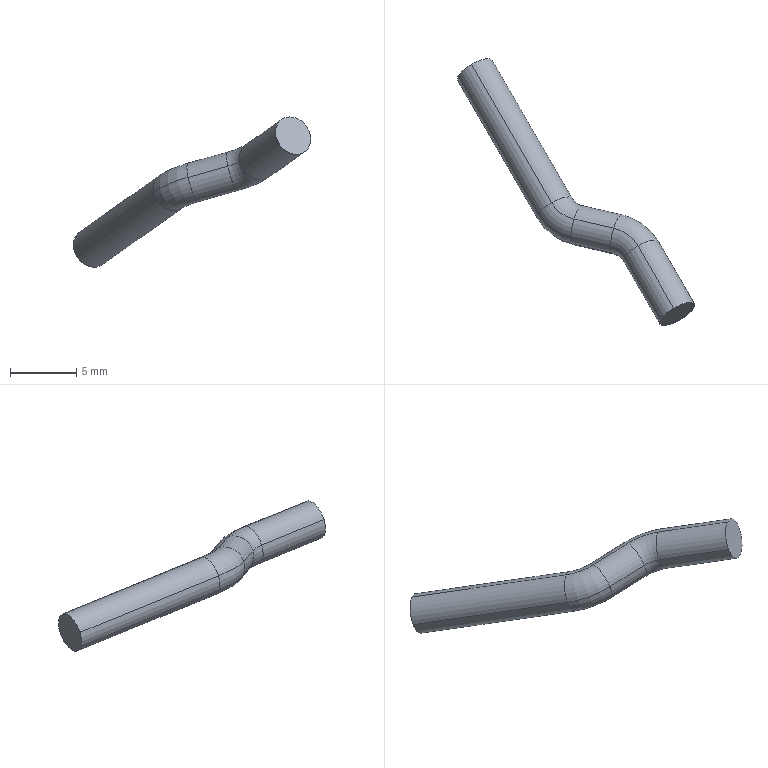Part | STEP file | MSBR-16_1_5_4_2_1 | 1 solid | 17 faces | box 17.856 x 20.083 x 11.306 mm | volume 186.454 mm3 | cylinder 9 | torus 6 | plane 2 | commonest cylinder face diameters 3 x9
STEP:
#1=CARTESIAN_POINT('',(0.,0.,0.));
#2=DIRECTION('',(0.,0.,1.));
#3=DIRECTION('',(1.,0.,0.));
#4=AXIS2_PLACEMENT_3D('',#1,#2,#3);
#5=CARTESIAN_POINT('',(6.735,-43.041,129.068));
#6=VERTEX_POINT('',#5);
#7=CARTESIAN_POINT('',(7.784,-41.858,130.482));
#8=VERTEX_POINT('',#7);
#9=CARTESIAN_POINT('',(8.034,-42.291,129.068));
#10=DIRECTION('',(-0.4714,0.8165,-0.3333));
#11=DIRECTION('',(-0.866,-0.5,-0.00009773));
#12=AXIS2_PLACEMENT_3D('',#9,#10,#11);
#13=CIRCLE('',#12,1.5);
#14=EDGE_CURVE('',#6,#8,#13,.T.);
#15=ORIENTED_EDGE('',*,*,#14,.F.);
#16=CARTESIAN_POINT('',(0.7209,-32.624,124.815));
#17=VERTEX_POINT('',#16);
#18=CARTESIAN_POINT('',(0.7209,-32.624,124.815));
#19=DIRECTION('',(0.4714,-0.8165,0.3333));
#20=VECTOR('',#19,12.757);
#21=LINE('',#18,#20);
#22=EDGE_CURVE('',#17,#6,#21,.T.);
#23=ORIENTED_EDGE('',*,*,#22,.F.);
#24=CARTESIAN_POINT('',(1.77,-31.441,126.23));
#25=VERTEX_POINT('',#24);
#26=CARTESIAN_POINT('',(2.02,-31.874,124.816));
#27=DIRECTION('',(0.4714,-0.8165,0.3333));
#28=DIRECTION('',(-0.1666,0.2887,0.9428));
#29=AXIS2_PLACEMENT_3D('',#26,#27,#28);
#30=CIRCLE('',#29,1.5);
#31=EDGE_CURVE('',#25,#17,#30,.T.);
#32=ORIENTED_EDGE('',*,*,#31,.F.);
#33=CARTESIAN_POINT('',(7.784,-41.858,130.482));
#34=DIRECTION('',(-0.4714,0.8165,-0.3333));
#35=VECTOR('',#34,12.757);
#36=LINE('',#33,#35);
#37=EDGE_CURVE('',#8,#25,#36,.T.);
#38=ORIENTED_EDGE('',*,*,#37,.F.);
#39=EDGE_LOOP('',(#15,#23,#32,#38));
#40=FACE_OUTER_BOUND('',#39,.F.);
#41=CARTESIAN_POINT('',(8.034,-42.291,129.068));
#42=DIRECTION('',(0.4714,-0.8165,0.3333));
#43=DIRECTION('',(-0.1668,0.2886,0.9428));
#44=AXIS2_PLACEMENT_3D('',#41,#42,#43);
#45=CYLINDRICAL_SURFACE('',#44,1.5);
#46=ADVANCED_FACE('',(#40),#45,.T.);
#47=CARTESIAN_POINT('',(9.468,-43.089,131.193));
#48=VERTEX_POINT('',#47);
#49=CARTESIAN_POINT('',(9.331,-44.939,130.163));
#50=VERTEX_POINT('',#49);
#51=CARTESIAN_POINT('',(9.753,-43.548,129.794));
#52=DIRECTION('',(0.9405,-0.2159,0.2624));
#53=DIRECTION('',(-0.1901,0.3058,0.9329));
#54=AXIS2_PLACEMENT_3D('',#51,#52,#53);
#55=CIRCLE('',#54,1.5);
#56=EDGE_CURVE('',#48,#50,#55,.T.);
#57=ORIENTED_EDGE('',*,*,#56,.T.);
#58=CARTESIAN_POINT('',(10.546,-40.772,129.236));
#59=DIRECTION('',(-0.2012,0.2684,0.9421));
#60=DIRECTION('',(-0.8587,-0.5112,-0.03777));
#61=AXIS2_PLACEMENT_3D('',#58,#59,#60);
#62=CIRCLE('',#61,4.439);
#63=EDGE_CURVE('',#6,#50,#62,.T.);
#64=ORIENTED_EDGE('',*,*,#63,.F.);
#65=ORIENTED_EDGE('',*,*,#14,.T.);
#66=CARTESIAN_POINT('',(10.257,-40.386,130.591));
#67=DIRECTION('',(0.2012,-0.2684,-0.9421));
#68=DIRECTION('',(-0.2738,-0.9388,0.209));
#69=AXIS2_PLACEMENT_3D('',#66,#67,#68);
#70=CIRCLE('',#69,2.88);
#71=EDGE_CURVE('',#48,#8,#70,.T.);
#72=ORIENTED_EDGE('',*,*,#71,.F.);
#73=EDGE_LOOP('',(#57,#64,#65,#72));
#74=FACE_OUTER_BOUND('',#73,.F.);
#75=CARTESIAN_POINT('',(10.558,-40.788,129.179));
#76=DIRECTION('',(0.2012,-0.2684,-0.9421));
#77=DIRECTION('',(-0.2738,-0.9388,0.209));
#78=AXIS2_PLACEMENT_3D('',#75,#76,#77);
#79=TOROIDAL_SURFACE('',#78,2.94,1.5);
#80=ADVANCED_FACE('',(#74),#79,.T.);
#81=CARTESIAN_POINT('',(12.313,-45.624,130.996));
#82=VERTEX_POINT('',#81);
#83=CARTESIAN_POINT('',(12.451,-43.774,132.025));
#84=VERTEX_POINT('',#83);
#85=CARTESIAN_POINT('',(12.736,-44.233,130.626));
#86=DIRECTION('',(-0.9405,0.2159,-0.2624));
#87=DIRECTION('',(-0.2817,-0.9273,0.2465));
#88=AXIS2_PLACEMENT_3D('',#85,#86,#87);
#89=CIRCLE('',#88,1.5);
#90=EDGE_CURVE('',#82,#84,#89,.T.);
#91=ORIENTED_EDGE('',*,*,#90,.F.);
#92=CARTESIAN_POINT('',(9.331,-44.939,130.163));
#93=DIRECTION('',(0.9405,-0.2159,0.2624));
#94=VECTOR('',#93,3.172);
#95=LINE('',#92,#94);
#96=EDGE_CURVE('',#50,#82,#95,.T.);
#97=ORIENTED_EDGE('',*,*,#96,.F.);
#98=ORIENTED_EDGE('',*,*,#56,.F.);
#99=CARTESIAN_POINT('',(12.451,-43.774,132.025));
#100=DIRECTION('',(-0.9405,0.2159,-0.2624));
#101=VECTOR('',#100,3.172);
#102=LINE('',#99,#101);
#103=EDGE_CURVE('',#84,#48,#102,.T.);
#104=ORIENTED_EDGE('',*,*,#103,.F.);
#105=EDGE_LOOP('',(#91,#97,#98,#104));
#106=FACE_OUTER_BOUND('',#105,.F.);
#107=CARTESIAN_POINT('',(12.736,-44.233,130.626));
#108=DIRECTION('',(0.9405,-0.2159,0.2624));
#109=DIRECTION('',(-0.1901,0.3057,0.933));
#110=AXIS2_PLACEMENT_3D('',#107,#108,#109);
#111=CYLINDRICAL_SURFACE('',#110,1.5);
#112=ADVANCED_FACE('',(#106),#111,.T.);
#113=CARTESIAN_POINT('',(14.276,-45.108,132.795));
#114=VERTEX_POINT('',#113);
#115=CARTESIAN_POINT('',(13.227,-46.291,131.381));
#116=VERTEX_POINT('',#115);
#117=CARTESIAN_POINT('',(14.526,-45.541,131.381));
#118=DIRECTION('',(0.4714,-0.8165,0.3333));
#119=DIRECTION('',(-0.1666,0.2887,0.9428));
#120=AXIS2_PLACEMENT_3D('',#117,#118,#119);
#121=CIRCLE('',#120,1.5);
#122=EDGE_CURVE('',#114,#116,#121,.T.);
#123=ORIENTED_EDGE('',*,*,#122,.T.);
#124=CARTESIAN_POINT('',(11.886,-47.089,131.322));
#125=DIRECTION('',(0.2012,-0.2684,-0.9421));
#126=DIRECTION('',(0.2738,0.9388,-0.209));
#127=AXIS2_PLACEMENT_3D('',#124,#125,#126);
#128=CIRCLE('',#127,1.561);
#129=EDGE_CURVE('',#82,#116,#128,.T.);
#130=ORIENTED_EDGE('',*,*,#129,.F.);
#131=ORIENTED_EDGE('',*,*,#90,.T.);
#132=CARTESIAN_POINT('',(11.596,-46.703,132.677));
#133=DIRECTION('',(-0.2012,0.2684,0.9421));
#134=DIRECTION('',(0.8587,0.5112,0.03777));
#135=AXIS2_PLACEMENT_3D('',#132,#133,#134);
#136=CIRCLE('',#135,3.12);
#137=EDGE_CURVE('',#114,#84,#136,.T.);
#138=ORIENTED_EDGE('',*,*,#137,.F.);
#139=EDGE_LOOP('',(#123,#130,#131,#138));
#140=FACE_OUTER_BOUND('',#139,.F.);
#141=CARTESIAN_POINT('',(11.898,-47.105,131.265));
#142=DIRECTION('',(-0.2012,0.2684,0.9421));
#143=DIRECTION('',(0.8587,0.5112,0.03777));
#144=AXIS2_PLACEMENT_3D('',#141,#142,#143);
#145=TOROIDAL_SURFACE('',#144,3.06,1.5);
#146=ADVANCED_FACE('',(#140),#145,.T.);
#147=CARTESIAN_POINT('',(15.931,-50.975,133.293));
#148=VERTEX_POINT('',#147);
#149=CARTESIAN_POINT('',(16.98,-49.792,134.707));
#150=VERTEX_POINT('',#149);
#151=CARTESIAN_POINT('',(17.23,-50.225,133.293));
#152=DIRECTION('',(-0.4714,0.8165,-0.3333));
#153=DIRECTION('',(-0.866,-0.5001,-0.0002609));
#154=AXIS2_PLACEMENT_3D('',#151,#152,#153);
#155=CIRCLE('',#154,1.5);
#156=EDGE_CURVE('',#148,#150,#155,.T.);
#157=ORIENTED_EDGE('',*,*,#156,.F.);
#158=CARTESIAN_POINT('',(13.227,-46.291,131.381));
#159=DIRECTION('',(0.4714,-0.8165,0.3333));
#160=VECTOR('',#159,5.737);
#161=LINE('',#158,#160);
#162=EDGE_CURVE('',#116,#148,#161,.T.);
#163=ORIENTED_EDGE('',*,*,#162,.F.);
#164=ORIENTED_EDGE('',*,*,#122,.F.);
#165=CARTESIAN_POINT('',(16.98,-49.792,134.707));
#166=DIRECTION('',(-0.4714,0.8165,-0.3333));
#167=VECTOR('',#166,5.737);
#168=LINE('',#165,#167);
#169=EDGE_CURVE('',#150,#114,#168,.T.);
#170=ORIENTED_EDGE('',*,*,#169,.F.);
#171=EDGE_LOOP('',(#157,#163,#164,#170));
#172=FACE_OUTER_BOUND('',#171,.F.);
#173=CARTESIAN_POINT('',(17.23,-50.225,133.293));
#174=DIRECTION('',(0.4714,-0.8165,0.3333));
#175=DIRECTION('',(-0.1668,0.2886,0.9428));
#176=AXIS2_PLACEMENT_3D('',#173,#174,#175);
#177=CYLINDRICAL_SURFACE('',#176,1.5);
#178=ADVANCED_FACE('',(#172),#177,.T.);
#179=CARTESIAN_POINT('',(18.529,-49.475,133.293));
#180=VERTEX_POINT('',#179);
#181=CARTESIAN_POINT('',(17.23,-50.225,133.293));
#182=DIRECTION('',(-0.4714,0.8165,-0.3333));
#183=DIRECTION('',(-0.1667,0.2886,0.9428));
#184=AXIS2_PLACEMENT_3D('',#181,#182,#183);
#185=CIRCLE('',#184,1.5);
#186=EDGE_CURVE('',#150,#180,#185,.T.);
#187=ORIENTED_EDGE('',*,*,#186,.T.);
#188=CARTESIAN_POINT('',(15.942,-50.992,133.236));
#189=VERTEX_POINT('',#188);
#190=CARTESIAN_POINT('',(17.23,-50.225,133.293));
#191=DIRECTION('',(-0.4714,0.8165,-0.3333));
#192=DIRECTION('',(0.866,0.5,0.00001838));
#193=AXIS2_PLACEMENT_3D('',#190,#191,#192);
#194=CIRCLE('',#193,1.5);
#195=EDGE_CURVE('',#180,#189,#194,.T.);
#196=ORIENTED_EDGE('',*,*,#195,.T.);
#197=CARTESIAN_POINT('',(17.23,-50.225,133.293));
#198=DIRECTION('',(-0.4714,0.8165,-0.3333));
#199=DIRECTION('',(-0.8587,-0.5112,-0.03777));
#200=AXIS2_PLACEMENT_3D('',#197,#198,#199);
#201=CIRCLE('',#200,1.5);
#202=EDGE_CURVE('',#189,#148,#201,.T.);
#203=ORIENTED_EDGE('',*,*,#202,.T.);
#204=ORIENTED_EDGE('',*,*,#156,.T.);
#205=EDGE_LOOP('',(#187,#196,#203,#204));
#206=FACE_OUTER_BOUND('',#205,.F.);
#207=CARTESIAN_POINT('',(17.178,-50.256,133.291));
#208=DIRECTION('',(-0.4714,0.8165,-0.3333));
#209=DIRECTION('',(-0.8587,-0.5112,-0.03777));
#210=AXIS2_PLACEMENT_3D('',#207,#208,#209);
#211=PLANE('',#210);
#212=ADVANCED_FACE('',(#206),#211,.F.);
#213=ORIENTED_EDGE('',*,*,#186,.F.);
#214=ORIENTED_EDGE('',*,*,#169,.T.);
#215=CARTESIAN_POINT('',(15.814,-44.775,131.438));
#216=VERTEX_POINT('',#215);
#217=CARTESIAN_POINT('',(14.526,-45.541,131.381));
#218=DIRECTION('',(0.4714,-0.8165,0.3333));
#219=DIRECTION('',(0.8587,0.5112,0.03777));
#220=AXIS2_PLACEMENT_3D('',#217,#218,#219);
#221=CIRCLE('',#220,1.5);
#222=EDGE_CURVE('',#216,#114,#221,.T.);
#223=ORIENTED_EDGE('',*,*,#222,.F.);
#224=CARTESIAN_POINT('',(15.825,-44.791,131.381));
#225=VERTEX_POINT('',#224);
#226=CARTESIAN_POINT('',(14.526,-45.541,131.381));
#227=DIRECTION('',(0.4714,-0.8165,0.3333));
#228=DIRECTION('',(0.866,0.5,-0.00001255));
#229=AXIS2_PLACEMENT_3D('',#226,#227,#228);
#230=CIRCLE('',#229,1.5);
#231=EDGE_CURVE('',#225,#216,#230,.T.);
#232=ORIENTED_EDGE('',*,*,#231,.F.);
#233=CARTESIAN_POINT('',(18.529,-49.475,133.293));
#234=DIRECTION('',(-0.4714,0.8165,-0.3333));
#235=VECTOR('',#234,5.737);
#236=LINE('',#233,#235);
#237=EDGE_CURVE('',#180,#225,#236,.T.);
#238=ORIENTED_EDGE('',*,*,#237,.F.);
#239=EDGE_LOOP('',(#213,#214,#223,#232,#238));
#240=FACE_OUTER_BOUND('',#239,.F.);
#241=CARTESIAN_POINT('',(17.23,-50.225,133.293));
#242=DIRECTION('',(0.4714,-0.8165,0.3333));
#243=DIRECTION('',(0.866,0.5,0.00009525));
#244=AXIS2_PLACEMENT_3D('',#241,#242,#243);
#245=CYLINDRICAL_SURFACE('',#244,1.5);
#246=ADVANCED_FACE('',(#240),#245,.T.);
#247=ORIENTED_EDGE('',*,*,#231,.T.);
#248=ORIENTED_EDGE('',*,*,#222,.T.);
#249=ORIENTED_EDGE('',*,*,#137,.T.);
#250=CARTESIAN_POINT('',(13.147,-42.824,130.312));
#251=VERTEX_POINT('',#250);
#252=CARTESIAN_POINT('',(12.736,-44.233,130.626));
#253=DIRECTION('',(-0.9405,0.2159,-0.2624));
#254=DIRECTION('',(-0.1901,0.3058,0.9329));
#255=AXIS2_PLACEMENT_3D('',#252,#253,#254);
#256=CIRCLE('',#255,1.5);
#257=EDGE_CURVE('',#84,#251,#256,.T.);
#258=ORIENTED_EDGE('',*,*,#257,.T.);
#259=CARTESIAN_POINT('',(13.158,-42.842,130.256));
#260=VERTEX_POINT('',#259);
#261=CARTESIAN_POINT('',(12.736,-44.233,130.626));
#262=DIRECTION('',(-0.9405,0.2159,-0.2624));
#263=DIRECTION('',(0.2738,0.9388,-0.209));
#264=AXIS2_PLACEMENT_3D('',#261,#262,#263);
#265=CIRCLE('',#264,1.5);
#266=EDGE_CURVE('',#251,#260,#265,.T.);
#267=ORIENTED_EDGE('',*,*,#266,.T.);
#268=CARTESIAN_POINT('',(11.91,-47.122,131.209));
#269=DIRECTION('',(-0.2012,0.2684,0.9421));
#270=DIRECTION('',(0.8587,0.5112,0.03777));
#271=AXIS2_PLACEMENT_3D('',#268,#269,#270);
#272=CIRCLE('',#271,4.559);
#273=EDGE_CURVE('',#225,#260,#272,.T.);
#274=ORIENTED_EDGE('',*,*,#273,.F.);
#275=EDGE_LOOP('',(#247,#248,#249,#258,#267,#274));
#276=FACE_OUTER_BOUND('',#275,.F.);
#277=CARTESIAN_POINT('',(11.898,-47.105,131.265));
#278=DIRECTION('',(-0.2012,0.2684,0.9421));
#279=DIRECTION('',(0.8587,0.5112,0.03777));
#280=AXIS2_PLACEMENT_3D('',#277,#278,#279);
#281=TOROIDAL_SURFACE('',#280,3.06,1.5);
#282=ADVANCED_FACE('',(#276),#281,.T.);
#283=ORIENTED_EDGE('',*,*,#266,.F.);
#284=ORIENTED_EDGE('',*,*,#257,.F.);
#285=ORIENTED_EDGE('',*,*,#103,.T.);
#286=CARTESIAN_POINT('',(10.164,-42.14,129.48));
#287=VERTEX_POINT('',#286);
#288=CARTESIAN_POINT('',(9.753,-43.548,129.793));
#289=DIRECTION('',(0.9405,-0.2159,0.2624));
#290=DIRECTION('',(0.2738,0.9388,-0.209));
#291=AXIS2_PLACEMENT_3D('',#288,#289,#290);
#292=CIRCLE('',#291,1.5);
#293=EDGE_CURVE('',#287,#48,#292,.T.);
#294=ORIENTED_EDGE('',*,*,#293,.F.);
#295=CARTESIAN_POINT('',(10.176,-42.157,129.424));
#296=VERTEX_POINT('',#295);
#297=CARTESIAN_POINT('',(9.753,-43.548,129.793));
#298=DIRECTION('',(0.9405,-0.2159,0.2624));
#299=DIRECTION('',(0.2817,0.9273,-0.2466));
#300=AXIS2_PLACEMENT_3D('',#297,#298,#299);
#301=CIRCLE('',#300,1.5);
#302=EDGE_CURVE('',#296,#287,#301,.T.);
#303=ORIENTED_EDGE('',*,*,#302,.F.);
#304=CARTESIAN_POINT('',(13.158,-42.842,130.256));
#305=DIRECTION('',(-0.9405,0.2159,-0.2624));
#306=VECTOR('',#305,3.172);
#307=LINE('',#304,#306);
#308=EDGE_CURVE('',#260,#296,#307,.T.);
#309=ORIENTED_EDGE('',*,*,#308,.F.);
#310=EDGE_LOOP('',(#283,#284,#285,#294,#303,#309));
#311=FACE_OUTER_BOUND('',#310,.F.);
#312=CARTESIAN_POINT('',(12.736,-44.233,130.626));
#313=DIRECTION('',(0.9405,-0.2159,0.2624));
#314=DIRECTION('',(0.2816,0.9273,-0.2465));
#315=AXIS2_PLACEMENT_3D('',#312,#313,#314);
#316=CYLINDRICAL_SURFACE('',#315,1.5);
#317=ADVANCED_FACE('',(#311),#316,.T.);
#318=ORIENTED_EDGE('',*,*,#302,.T.);
#319=ORIENTED_EDGE('',*,*,#293,.T.);
#320=ORIENTED_EDGE('',*,*,#71,.T.);
#321=CARTESIAN_POINT('',(9.322,-41.524,129.125));
#322=VERTEX_POINT('',#321);
#323=CARTESIAN_POINT('',(8.034,-42.291,129.068));
#324=DIRECTION('',(-0.4714,0.8165,-0.3333));
#325=DIRECTION('',(-0.1667,0.2887,0.9428));
#326=AXIS2_PLACEMENT_3D('',#323,#324,#325);
#327=CIRCLE('',#326,1.5);
#328=EDGE_CURVE('',#8,#322,#327,.T.);
#329=ORIENTED_EDGE('',*,*,#328,.T.);
#330=CARTESIAN_POINT('',(9.333,-41.541,129.068));
#331=VERTEX_POINT('',#330);
#332=CARTESIAN_POINT('',(8.034,-42.291,129.068));
#333=DIRECTION('',(-0.4714,0.8165,-0.3333));
#334=DIRECTION('',(0.8587,0.5112,0.03777));
#335=AXIS2_PLACEMENT_3D('',#332,#333,#334);
#336=CIRCLE('',#335,1.5);
#337=EDGE_CURVE('',#322,#331,#336,.T.);
#338=ORIENTED_EDGE('',*,*,#337,.T.);
#339=CARTESIAN_POINT('',(10.57,-40.804,129.122));
#340=DIRECTION('',(0.2012,-0.2684,-0.9421));
#341=DIRECTION('',(-0.2738,-0.9388,0.209));
#342=AXIS2_PLACEMENT_3D('',#339,#340,#341);
#343=CIRCLE('',#342,1.441);
#344=EDGE_CURVE('',#296,#331,#343,.T.);
#345=ORIENTED_EDGE('',*,*,#344,.F.);
#346=EDGE_LOOP('',(#318,#319,#320,#329,#338,#345));
#347=FACE_OUTER_BOUND('',#346,.F.);
#348=CARTESIAN_POINT('',(10.558,-40.788,129.179));
#349=DIRECTION('',(0.2012,-0.2684,-0.9421));
#350=DIRECTION('',(-0.2738,-0.9388,0.209));
#351=AXIS2_PLACEMENT_3D('',#348,#349,#350);
#352=TOROIDAL_SURFACE('',#351,2.94,1.5);
#353=ADVANCED_FACE('',(#347),#352,.T.);
#354=ORIENTED_EDGE('',*,*,#337,.F.);
#355=ORIENTED_EDGE('',*,*,#328,.F.);
#356=ORIENTED_EDGE('',*,*,#37,.T.);
#357=CARTESIAN_POINT('',(3.319,-31.124,124.816));
#358=VERTEX_POINT('',#357);
#359=CARTESIAN_POINT('',(2.02,-31.874,124.816));
#360=DIRECTION('',(0.4714,-0.8165,0.3333));
#361=DIRECTION('',(0.866,0.5,-0.00003593));
#362=AXIS2_PLACEMENT_3D('',#359,#360,#361);
#363=CIRCLE('',#362,1.5);
#364=EDGE_CURVE('',#358,#25,#363,.T.);
#365=ORIENTED_EDGE('',*,*,#364,.F.);
#366=CARTESIAN_POINT('',(9.333,-41.541,129.068));
#367=DIRECTION('',(-0.4714,0.8165,-0.3333));
#368=VECTOR('',#367,12.757);
#369=LINE('',#366,#368);
#370=EDGE_CURVE('',#331,#358,#369,.T.);
#371=ORIENTED_EDGE('',*,*,#370,.F.);
#372=EDGE_LOOP('',(#354,#355,#356,#365,#371));
#373=FACE_OUTER_BOUND('',#372,.F.);
#374=CARTESIAN_POINT('',(8.034,-42.291,129.068));
#375=DIRECTION('',(0.4714,-0.8165,0.3333));
#376=DIRECTION('',(0.866,0.5,0.00009525));
#377=AXIS2_PLACEMENT_3D('',#374,#375,#376);
#378=CYLINDRICAL_SURFACE('',#377,1.5);
#379=ADVANCED_FACE('',(#373),#378,.T.);
#380=ORIENTED_EDGE('',*,*,#364,.T.);
#381=ORIENTED_EDGE('',*,*,#31,.T.);
#382=CARTESIAN_POINT('',(0.7319,-32.641,124.759));
#383=VERTEX_POINT('',#382);
#384=CARTESIAN_POINT('',(2.02,-31.874,124.816));
#385=DIRECTION('',(0.4714,-0.8165,0.3333));
#386=DIRECTION('',(-0.866,-0.5001,-0.0002071));
#387=AXIS2_PLACEMENT_3D('',#384,#385,#386);
#388=CIRCLE('',#387,1.5);
#389=EDGE_CURVE('',#17,#383,#388,.T.);
#390=ORIENTED_EDGE('',*,*,#389,.T.);
#391=CARTESIAN_POINT('',(2.02,-31.874,124.816));
#392=DIRECTION('',(0.4714,-0.8165,0.3333));
#393=DIRECTION('',(-0.8587,-0.5112,-0.03777));
#394=AXIS2_PLACEMENT_3D('',#391,#392,#393);
#395=CIRCLE('',#394,1.5);
#396=EDGE_CURVE('',#383,#358,#395,.T.);
#397=ORIENTED_EDGE('',*,*,#396,.T.);
#398=EDGE_LOOP('',(#380,#381,#390,#397));
#399=FACE_OUTER_BOUND('',#398,.F.);
#400=CARTESIAN_POINT('',(1.968,-31.905,124.813));
#401=DIRECTION('',(-0.4714,0.8165,-0.3333));
#402=DIRECTION('',(-0.8587,-0.5112,-0.03777));
#403=AXIS2_PLACEMENT_3D('',#400,#401,#402);
#404=PLANE('',#403);
#405=ADVANCED_FACE('',(#399),#404,.T.);
#406=CARTESIAN_POINT('',(6.746,-43.057,129.011));
#407=VERTEX_POINT('',#406);
#408=CARTESIAN_POINT('',(8.034,-42.291,129.068));
#409=DIRECTION('',(-0.4714,0.8165,-0.3333));
#410=DIRECTION('',(-0.8587,-0.5112,-0.03777));
#411=AXIS2_PLACEMENT_3D('',#408,#409,#410);
#412=CIRCLE('',#411,1.5);
#413=EDGE_CURVE('',#407,#6,#412,.T.);
#414=ORIENTED_EDGE('',*,*,#413,.F.);
#415=CARTESIAN_POINT('',(8.034,-42.291,129.068));
#416=DIRECTION('',(-0.4714,0.8165,-0.3333));
#417=DIRECTION('',(0.866,0.5,-0.000009486));
#418=AXIS2_PLACEMENT_3D('',#415,#416,#417);
#419=CIRCLE('',#418,1.5);
#420=EDGE_CURVE('',#331,#407,#419,.T.);
#421=ORIENTED_EDGE('',*,*,#420,.F.);
#422=ORIENTED_EDGE('',*,*,#370,.T.);
#423=ORIENTED_EDGE('',*,*,#396,.F.);
#424=ORIENTED_EDGE('',*,*,#389,.F.);
#425=ORIENTED_EDGE('',*,*,#22,.T.);
#426=EDGE_LOOP('',(#414,#421,#422,#423,#424,#425));
#427=FACE_OUTER_BOUND('',#426,.F.);
#428=CARTESIAN_POINT('',(8.034,-42.291,129.068));
#429=DIRECTION('',(-0.4714,0.8165,-0.3333));
#430=DIRECTION('',(-0.8587,-0.5112,-0.03777));
#431=AXIS2_PLACEMENT_3D('',#428,#429,#430);
#432=CYLINDRICAL_SURFACE('',#431,1.5);
#433=ADVANCED_FACE('',(#427),#432,.T.);
#434=CARTESIAN_POINT('',(9.342,-44.956,130.107));
#435=VERTEX_POINT('',#434);
#436=CARTESIAN_POINT('',(9.753,-43.548,129.793));
#437=DIRECTION('',(0.9405,-0.2159,0.2624));
#438=DIRECTION('',(-0.2817,-0.9273,0.2465));
#439=AXIS2_PLACEMENT_3D('',#436,#437,#438);
#440=CIRCLE('',#439,1.5);
#441=EDGE_CURVE('',#50,#435,#440,.T.);
#442=ORIENTED_EDGE('',*,*,#441,.T.);
#443=CARTESIAN_POINT('',(9.753,-43.548,129.793));
#444=DIRECTION('',(0.9405,-0.2159,0.2624));
#445=DIRECTION('',(-0.2738,-0.9388,0.209));
#446=AXIS2_PLACEMENT_3D('',#443,#444,#445);
#447=CIRCLE('',#446,1.5);
#448=EDGE_CURVE('',#435,#296,#447,.T.);
#449=ORIENTED_EDGE('',*,*,#448,.T.);
#450=ORIENTED_EDGE('',*,*,#344,.T.);
#451=ORIENTED_EDGE('',*,*,#420,.T.);
#452=ORIENTED_EDGE('',*,*,#413,.T.);
#453=ORIENTED_EDGE('',*,*,#63,.T.);
#454=EDGE_LOOP('',(#442,#449,#450,#451,#452,#453));
#455=FACE_OUTER_BOUND('',#454,.F.);
#456=CARTESIAN_POINT('',(10.558,-40.788,129.179));
#457=DIRECTION('',(0.2012,-0.2684,-0.9421));
#458=DIRECTION('',(0.2738,0.9388,-0.209));
#459=AXIS2_PLACEMENT_3D('',#456,#457,#458);
#460=TOROIDAL_SURFACE('',#459,2.94,1.5);
#461=ADVANCED_FACE('',(#455),#460,.T.);
#462=CARTESIAN_POINT('',(12.325,-45.641,130.939));
#463=VERTEX_POINT('',#462);
#464=CARTESIAN_POINT('',(12.736,-44.233,130.626));
#465=DIRECTION('',(-0.9405,0.2159,-0.2624));
#466=DIRECTION('',(-0.2738,-0.9388,0.209));
#467=AXIS2_PLACEMENT_3D('',#464,#465,#466);
#468=CIRCLE('',#467,1.5);
#469=EDGE_CURVE('',#463,#82,#468,.T.);
#470=ORIENTED_EDGE('',*,*,#469,.F.);
#471=CARTESIAN_POINT('',(12.736,-44.233,130.626));
#472=DIRECTION('',(-0.9405,0.2159,-0.2624));
#473=DIRECTION('',(0.2817,0.9273,-0.2466));
#474=AXIS2_PLACEMENT_3D('',#471,#472,#473);
#475=CIRCLE('',#474,1.5);
#476=EDGE_CURVE('',#260,#463,#475,.T.);
#477=ORIENTED_EDGE('',*,*,#476,.F.);
#478=ORIENTED_EDGE('',*,*,#308,.T.);
#479=ORIENTED_EDGE('',*,*,#448,.F.);
#480=ORIENTED_EDGE('',*,*,#441,.F.);
#481=ORIENTED_EDGE('',*,*,#96,.T.);
#482=EDGE_LOOP('',(#470,#477,#478,#479,#480,#481));
#483=FACE_OUTER_BOUND('',#482,.F.);
#484=CARTESIAN_POINT('',(12.736,-44.233,130.626));
#485=DIRECTION('',(-0.9405,0.2159,-0.2624));
#486=DIRECTION('',(-0.2738,-0.9388,0.209));
#487=AXIS2_PLACEMENT_3D('',#484,#485,#486);
#488=CYLINDRICAL_SURFACE('',#487,1.5);
#489=ADVANCED_FACE('',(#483),#488,.T.);
#490=CARTESIAN_POINT('',(13.238,-46.308,131.324));
#491=VERTEX_POINT('',#490);
#492=CARTESIAN_POINT('',(14.526,-45.541,131.381));
#493=DIRECTION('',(0.4714,-0.8165,0.3333));
#494=DIRECTION('',(-0.866,-0.5,-0.00007266));
#495=AXIS2_PLACEMENT_3D('',#492,#493,#494);
#496=CIRCLE('',#495,1.5);
#497=EDGE_CURVE('',#116,#491,#496,.T.);
#498=ORIENTED_EDGE('',*,*,#497,.T.);
#499=CARTESIAN_POINT('',(14.526,-45.541,131.381));
#500=DIRECTION('',(0.4714,-0.8165,0.3333));
#501=DIRECTION('',(-0.8587,-0.5112,-0.03777));
#502=AXIS2_PLACEMENT_3D('',#499,#500,#501);
#503=CIRCLE('',#502,1.5);
#504=EDGE_CURVE('',#491,#225,#503,.T.);
#505=ORIENTED_EDGE('',*,*,#504,.T.);
#506=ORIENTED_EDGE('',*,*,#273,.T.);
#507=ORIENTED_EDGE('',*,*,#476,.T.);
#508=ORIENTED_EDGE('',*,*,#469,.T.);
#509=ORIENTED_EDGE('',*,*,#129,.T.);
#510=EDGE_LOOP('',(#498,#505,#506,#507,#508,#509));
#511=FACE_OUTER_BOUND('',#510,.F.);
#512=CARTESIAN_POINT('',(11.898,-47.105,131.265));
#513=DIRECTION('',(-0.2012,0.2684,0.9421));
#514=DIRECTION('',(-0.8587,-0.5112,-0.03777));
#515=AXIS2_PLACEMENT_3D('',#512,#513,#514);
#516=TOROIDAL_SURFACE('',#515,3.06,1.5);
#517=ADVANCED_FACE('',(#511),#516,.T.);
#518=ORIENTED_EDGE('',*,*,#202,.F.);
#519=ORIENTED_EDGE('',*,*,#195,.F.);
#520=ORIENTED_EDGE('',*,*,#237,.T.);
#521=ORIENTED_EDGE('',*,*,#504,.F.);
#522=ORIENTED_EDGE('',*,*,#497,.F.);
#523=ORIENTED_EDGE('',*,*,#162,.T.);
#524=EDGE_LOOP('',(#518,#519,#520,#521,#522,#523));
#525=FACE_OUTER_BOUND('',#524,.F.);
#526=CARTESIAN_POINT('',(17.23,-50.225,133.293));
#527=DIRECTION('',(-0.4714,0.8165,-0.3333));
#528=DIRECTION('',(-0.8587,-0.5112,-0.03777));
#529=AXIS2_PLACEMENT_3D('',#526,#527,#528);
#530=CYLINDRICAL_SURFACE('',#529,1.5);
#531=ADVANCED_FACE('',(#525),#530,.T.);
#532=CLOSED_SHELL('',(#46,#80,#112,#146,#178,#212,#246,#282,#317,#353,#379,#405,#433,#461,#489,#517,#531));
#533=MANIFOLD_SOLID_BREP('',#532);
#534=(LENGTH_UNIT()NAMED_UNIT(*)SI_UNIT(.MILLI.,.METRE.));
#535=UNCERTAINTY_MEASURE_WITH_UNIT(LENGTH_MEASURE(0.002994),#534,'','');
#536=(NAMED_UNIT(*)PLANE_ANGLE_UNIT()SI_UNIT($,.RADIAN.));
#537=PLANE_ANGLE_MEASURE_WITH_UNIT(PLANE_ANGLE_MEASURE(0.01745),#536);
#538=(CONVERSION_BASED_UNIT('DEGREE',#537)NAMED_UNIT(*)PLANE_ANGLE_UNIT());
#539=(NAMED_UNIT(*)SI_UNIT($,.STERADIAN.)SOLID_ANGLE_UNIT());
#540=(GEOMETRIC_REPRESENTATION_CONTEXT(3)GLOBAL_UNCERTAINTY_ASSIGNED_CONTEXT((#535))GLOBAL_UNIT_ASSIGNED_CONTEXT((#534,#538,#539))REPRESENTATION_CONTEXT('',''));
#541=ADVANCED_BREP_SHAPE_REPRESENTATION('',(#4,#533),#540);